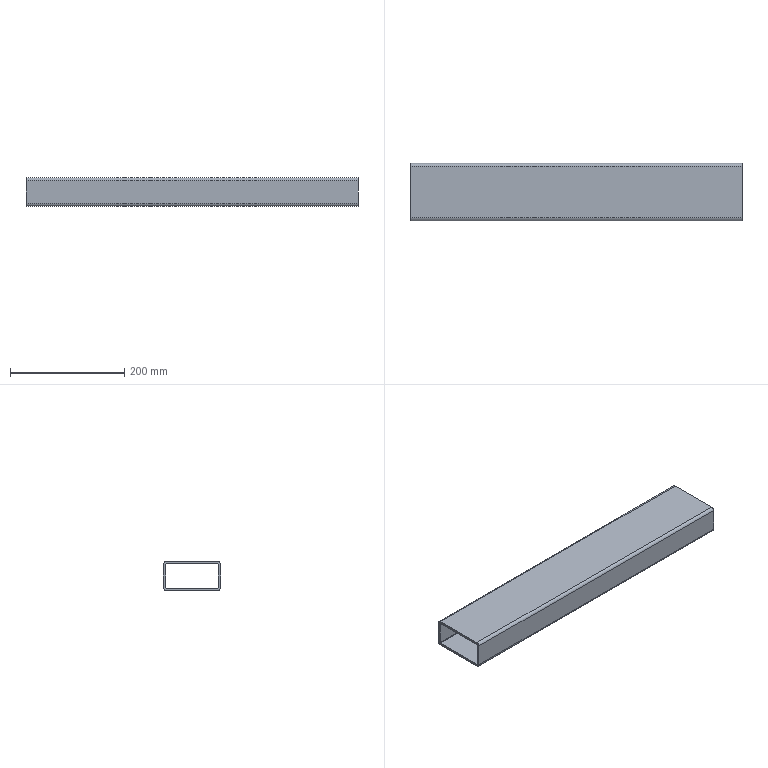Part | SolidWorks | features BaseBody 1 | 1 solid | 18 faces | box 580 x 100 x 50 mm | volume 646931 mm3 | plane 10 | cylinder 8 | commonest cylinder face diameters 2 x4 10 x4
STEP:
#1=CARTESIAN_POINT('',(-290.,45.,-25.));
#2=VERTEX_POINT('',#1);
#3=CARTESIAN_POINT('',(-290.,50.,-20.));
#4=VERTEX_POINT('',#3);
#5=CARTESIAN_POINT('',(-290.,45.,-20.));
#6=DIRECTION('',(1.,0.,0.));
#7=DIRECTION('',(0.,0.,-1.));
#8=AXIS2_PLACEMENT_3D('',#5,#6,#7);
#9=CIRCLE('',#8,5.);
#10=EDGE_CURVE('',#2,#4,#9,.T.);
#11=ORIENTED_EDGE('',*,*,#10,.T.);
#12=CARTESIAN_POINT('',(290.,50.,-20.));
#13=VERTEX_POINT('',#12);
#14=CARTESIAN_POINT('',(290.,50.,-20.));
#15=DIRECTION('',(-1.,0.,0.));
#16=VECTOR('',#15,1000.);
#17=LINE('',#14,#16);
#18=EDGE_CURVE('',#13,#4,#17,.T.);
#19=ORIENTED_EDGE('',*,*,#18,.F.);
#20=CARTESIAN_POINT('',(290.,45.,-25.));
#21=VERTEX_POINT('',#20);
#22=CARTESIAN_POINT('',(290.,45.,-20.));
#23=DIRECTION('',(1.,0.,0.));
#24=DIRECTION('',(0.,0.,-1.));
#25=AXIS2_PLACEMENT_3D('',#22,#23,#24);
#26=CIRCLE('',#25,5.);
#27=EDGE_CURVE('',#21,#13,#26,.T.);
#28=ORIENTED_EDGE('',*,*,#27,.F.);
#29=CARTESIAN_POINT('',(290.,45.,-25.));
#30=DIRECTION('',(-1.,0.,0.));
#31=VECTOR('',#30,1000.);
#32=LINE('',#29,#31);
#33=EDGE_CURVE('',#21,#2,#32,.T.);
#34=ORIENTED_EDGE('',*,*,#33,.T.);
#35=EDGE_LOOP('',(#11,#19,#28,#34));
#36=FACE_OUTER_BOUND('',#35,.T.);
#37=CARTESIAN_POINT('',(290.,45.,-20.));
#38=DIRECTION('',(-1.,0.,0.));
#39=DIRECTION('',(0.,0.,1.));
#40=AXIS2_PLACEMENT_3D('',#37,#38,#39);
#41=CYLINDRICAL_SURFACE('',#40,5.);
#42=ADVANCED_FACE('',(#36),#41,.T.);
#43=CARTESIAN_POINT('',(-290.,50.,20.));
#44=VERTEX_POINT('',#43);
#45=CARTESIAN_POINT('',(-290.,50.,-20.));
#46=DIRECTION('',(0.,0.,1.));
#47=VECTOR('',#46,1000.);
#48=LINE('',#45,#47);
#49=EDGE_CURVE('',#4,#44,#48,.T.);
#50=ORIENTED_EDGE('',*,*,#49,.T.);
#51=CARTESIAN_POINT('',(290.,50.,20.));
#52=VERTEX_POINT('',#51);
#53=CARTESIAN_POINT('',(290.,50.,20.));
#54=DIRECTION('',(-1.,0.,0.));
#55=VECTOR('',#54,1000.);
#56=LINE('',#53,#55);
#57=EDGE_CURVE('',#52,#44,#56,.T.);
#58=ORIENTED_EDGE('',*,*,#57,.F.);
#59=CARTESIAN_POINT('',(290.,50.,-20.));
#60=DIRECTION('',(0.,0.,1.));
#61=VECTOR('',#60,1000.);
#62=LINE('',#59,#61);
#63=EDGE_CURVE('',#13,#52,#62,.T.);
#64=ORIENTED_EDGE('',*,*,#63,.F.);
#65=ORIENTED_EDGE('',*,*,#18,.T.);
#66=EDGE_LOOP('',(#50,#58,#64,#65));
#67=FACE_OUTER_BOUND('',#66,.T.);
#68=CARTESIAN_POINT('',(290.,50.,-20.));
#69=DIRECTION('',(0.,-1.,0.));
#70=DIRECTION('',(0.,0.,-1.));
#71=AXIS2_PLACEMENT_3D('',#68,#69,#70);
#72=PLANE('',#71);
#73=ADVANCED_FACE('',(#67),#72,.F.);
#74=CARTESIAN_POINT('',(-290.,45.,25.));
#75=VERTEX_POINT('',#74);
#76=CARTESIAN_POINT('',(-290.,45.,20.));
#77=DIRECTION('',(1.,0.,0.));
#78=DIRECTION('',(0.,0.,-1.));
#79=AXIS2_PLACEMENT_3D('',#76,#77,#78);
#80=CIRCLE('',#79,5.);
#81=EDGE_CURVE('',#44,#75,#80,.T.);
#82=ORIENTED_EDGE('',*,*,#81,.T.);
#83=CARTESIAN_POINT('',(290.,45.,25.));
#84=VERTEX_POINT('',#83);
#85=CARTESIAN_POINT('',(290.,45.,25.));
#86=DIRECTION('',(-1.,0.,0.));
#87=VECTOR('',#86,1000.);
#88=LINE('',#85,#87);
#89=EDGE_CURVE('',#84,#75,#88,.T.);
#90=ORIENTED_EDGE('',*,*,#89,.F.);
#91=CARTESIAN_POINT('',(290.,45.,20.));
#92=DIRECTION('',(1.,0.,0.));
#93=DIRECTION('',(0.,0.,-1.));
#94=AXIS2_PLACEMENT_3D('',#91,#92,#93);
#95=CIRCLE('',#94,5.);
#96=EDGE_CURVE('',#52,#84,#95,.T.);
#97=ORIENTED_EDGE('',*,*,#96,.F.);
#98=ORIENTED_EDGE('',*,*,#57,.T.);
#99=EDGE_LOOP('',(#82,#90,#97,#98));
#100=FACE_OUTER_BOUND('',#99,.T.);
#101=CARTESIAN_POINT('',(290.,45.,20.));
#102=DIRECTION('',(-1.,0.,0.));
#103=DIRECTION('',(0.,0.,1.));
#104=AXIS2_PLACEMENT_3D('',#101,#102,#103);
#105=CYLINDRICAL_SURFACE('',#104,5.);
#106=ADVANCED_FACE('',(#100),#105,.T.);
#107=CARTESIAN_POINT('',(-290.,-45.,25.));
#108=VERTEX_POINT('',#107);
#109=CARTESIAN_POINT('',(-290.,-45.,25.));
#110=DIRECTION('',(0.,-1.,0.));
#111=VECTOR('',#110,1000.);
#112=LINE('',#109,#111);
#113=EDGE_CURVE('',#75,#108,#112,.T.);
#114=ORIENTED_EDGE('',*,*,#113,.T.);
#115=CARTESIAN_POINT('',(290.,-45.,25.));
#116=VERTEX_POINT('',#115);
#117=CARTESIAN_POINT('',(290.,-45.,25.));
#118=DIRECTION('',(-1.,0.,0.));
#119=VECTOR('',#118,1000.);
#120=LINE('',#117,#119);
#121=EDGE_CURVE('',#116,#108,#120,.T.);
#122=ORIENTED_EDGE('',*,*,#121,.F.);
#123=CARTESIAN_POINT('',(290.,-45.,25.));
#124=DIRECTION('',(0.,-1.,0.));
#125=VECTOR('',#124,1000.);
#126=LINE('',#123,#125);
#127=EDGE_CURVE('',#84,#116,#126,.T.);
#128=ORIENTED_EDGE('',*,*,#127,.F.);
#129=ORIENTED_EDGE('',*,*,#89,.T.);
#130=EDGE_LOOP('',(#114,#122,#128,#129));
#131=FACE_OUTER_BOUND('',#130,.T.);
#132=CARTESIAN_POINT('',(290.,-45.,25.));
#133=DIRECTION('',(0.,0.,-1.));
#134=DIRECTION('',(0.,1.,0.));
#135=AXIS2_PLACEMENT_3D('',#132,#133,#134);
#136=PLANE('',#135);
#137=ADVANCED_FACE('',(#131),#136,.F.);
#138=CARTESIAN_POINT('',(-290.,-50.,20.));
#139=VERTEX_POINT('',#138);
#140=CARTESIAN_POINT('',(-290.,-45.,20.));
#141=DIRECTION('',(1.,0.,0.));
#142=DIRECTION('',(0.,0.,-1.));
#143=AXIS2_PLACEMENT_3D('',#140,#141,#142);
#144=CIRCLE('',#143,5.);
#145=EDGE_CURVE('',#108,#139,#144,.T.);
#146=ORIENTED_EDGE('',*,*,#145,.T.);
#147=CARTESIAN_POINT('',(290.,-50.,20.));
#148=VERTEX_POINT('',#147);
#149=CARTESIAN_POINT('',(290.,-50.,20.));
#150=DIRECTION('',(-1.,0.,0.));
#151=VECTOR('',#150,1000.);
#152=LINE('',#149,#151);
#153=EDGE_CURVE('',#148,#139,#152,.T.);
#154=ORIENTED_EDGE('',*,*,#153,.F.);
#155=CARTESIAN_POINT('',(290.,-45.,20.));
#156=DIRECTION('',(1.,0.,0.));
#157=DIRECTION('',(0.,0.,-1.));
#158=AXIS2_PLACEMENT_3D('',#155,#156,#157);
#159=CIRCLE('',#158,5.);
#160=EDGE_CURVE('',#116,#148,#159,.T.);
#161=ORIENTED_EDGE('',*,*,#160,.F.);
#162=ORIENTED_EDGE('',*,*,#121,.T.);
#163=EDGE_LOOP('',(#146,#154,#161,#162));
#164=FACE_OUTER_BOUND('',#163,.T.);
#165=CARTESIAN_POINT('',(290.,-45.,20.));
#166=DIRECTION('',(-1.,0.,0.));
#167=DIRECTION('',(0.,0.,1.));
#168=AXIS2_PLACEMENT_3D('',#165,#166,#167);
#169=CYLINDRICAL_SURFACE('',#168,5.);
#170=ADVANCED_FACE('',(#164),#169,.T.);
#171=CARTESIAN_POINT('',(-290.,-50.,-20.));
#172=VERTEX_POINT('',#171);
#173=CARTESIAN_POINT('',(-290.,-50.,20.));
#174=DIRECTION('',(0.,0.,-1.));
#175=VECTOR('',#174,1000.);
#176=LINE('',#173,#175);
#177=EDGE_CURVE('',#139,#172,#176,.T.);
#178=ORIENTED_EDGE('',*,*,#177,.T.);
#179=CARTESIAN_POINT('',(290.,-50.,-20.));
#180=VERTEX_POINT('',#179);
#181=CARTESIAN_POINT('',(290.,-50.,-20.));
#182=DIRECTION('',(-1.,0.,0.));
#183=VECTOR('',#182,1000.);
#184=LINE('',#181,#183);
#185=EDGE_CURVE('',#180,#172,#184,.T.);
#186=ORIENTED_EDGE('',*,*,#185,.F.);
#187=CARTESIAN_POINT('',(290.,-50.,20.));
#188=DIRECTION('',(0.,0.,-1.));
#189=VECTOR('',#188,1000.);
#190=LINE('',#187,#189);
#191=EDGE_CURVE('',#148,#180,#190,.T.);
#192=ORIENTED_EDGE('',*,*,#191,.F.);
#193=ORIENTED_EDGE('',*,*,#153,.T.);
#194=EDGE_LOOP('',(#178,#186,#192,#193));
#195=FACE_OUTER_BOUND('',#194,.T.);
#196=CARTESIAN_POINT('',(290.,-50.,20.));
#197=DIRECTION('',(0.,1.,0.));
#198=DIRECTION('',(0.,0.,1.));
#199=AXIS2_PLACEMENT_3D('',#196,#197,#198);
#200=PLANE('',#199);
#201=ADVANCED_FACE('',(#195),#200,.F.);
#202=CARTESIAN_POINT('',(-290.,-45.,-25.));
#203=VERTEX_POINT('',#202);
#204=CARTESIAN_POINT('',(-290.,-45.,-20.));
#205=DIRECTION('',(1.,0.,0.));
#206=DIRECTION('',(0.,0.,-1.));
#207=AXIS2_PLACEMENT_3D('',#204,#205,#206);
#208=CIRCLE('',#207,5.);
#209=EDGE_CURVE('',#172,#203,#208,.T.);
#210=ORIENTED_EDGE('',*,*,#209,.T.);
#211=CARTESIAN_POINT('',(290.,-45.,-25.));
#212=VERTEX_POINT('',#211);
#213=CARTESIAN_POINT('',(290.,-45.,-25.));
#214=DIRECTION('',(-1.,0.,0.));
#215=VECTOR('',#214,1000.);
#216=LINE('',#213,#215);
#217=EDGE_CURVE('',#212,#203,#216,.T.);
#218=ORIENTED_EDGE('',*,*,#217,.F.);
#219=CARTESIAN_POINT('',(290.,-45.,-20.));
#220=DIRECTION('',(1.,0.,0.));
#221=DIRECTION('',(0.,0.,-1.));
#222=AXIS2_PLACEMENT_3D('',#219,#220,#221);
#223=CIRCLE('',#222,5.);
#224=EDGE_CURVE('',#180,#212,#223,.T.);
#225=ORIENTED_EDGE('',*,*,#224,.F.);
#226=ORIENTED_EDGE('',*,*,#185,.T.);
#227=EDGE_LOOP('',(#210,#218,#225,#226));
#228=FACE_OUTER_BOUND('',#227,.T.);
#229=CARTESIAN_POINT('',(290.,-45.,-20.));
#230=DIRECTION('',(-1.,0.,0.));
#231=DIRECTION('',(0.,0.,1.));
#232=AXIS2_PLACEMENT_3D('',#229,#230,#231);
#233=CYLINDRICAL_SURFACE('',#232,5.);
#234=ADVANCED_FACE('',(#228),#233,.T.);
#235=CARTESIAN_POINT('',(-290.,46.,20.));
#236=VERTEX_POINT('',#235);
#237=CARTESIAN_POINT('',(-290.,45.,21.));
#238=VERTEX_POINT('',#237);
#239=CARTESIAN_POINT('',(-290.,45.,20.));
#240=DIRECTION('',(1.,0.,0.));
#241=DIRECTION('',(0.,0.,-1.));
#242=AXIS2_PLACEMENT_3D('',#239,#240,#241);
#243=CIRCLE('',#242,1.);
#244=EDGE_CURVE('',#236,#238,#243,.T.);
#245=ORIENTED_EDGE('',*,*,#244,.F.);
#246=CARTESIAN_POINT('',(290.,46.,20.));
#247=VERTEX_POINT('',#246);
#248=CARTESIAN_POINT('',(290.,46.,20.));
#249=DIRECTION('',(-1.,0.,0.));
#250=VECTOR('',#249,1000.);
#251=LINE('',#248,#250);
#252=EDGE_CURVE('',#247,#236,#251,.T.);
#253=ORIENTED_EDGE('',*,*,#252,.F.);
#254=CARTESIAN_POINT('',(290.,45.,21.));
#255=VERTEX_POINT('',#254);
#256=CARTESIAN_POINT('',(290.,45.,20.));
#257=DIRECTION('',(1.,0.,0.));
#258=DIRECTION('',(0.,0.,-1.));
#259=AXIS2_PLACEMENT_3D('',#256,#257,#258);
#260=CIRCLE('',#259,1.);
#261=EDGE_CURVE('',#247,#255,#260,.T.);
#262=ORIENTED_EDGE('',*,*,#261,.T.);
#263=CARTESIAN_POINT('',(290.,45.,21.));
#264=DIRECTION('',(-1.,0.,0.));
#265=VECTOR('',#264,1000.);
#266=LINE('',#263,#265);
#267=EDGE_CURVE('',#255,#238,#266,.T.);
#268=ORIENTED_EDGE('',*,*,#267,.T.);
#269=EDGE_LOOP('',(#245,#253,#262,#268));
#270=FACE_OUTER_BOUND('',#269,.T.);
#271=CARTESIAN_POINT('',(290.,45.,20.));
#272=DIRECTION('',(-1.,0.,0.));
#273=DIRECTION('',(0.,0.,1.));
#274=AXIS2_PLACEMENT_3D('',#271,#272,#273);
#275=CYLINDRICAL_SURFACE('',#274,1.);
#276=ADVANCED_FACE('',(#270),#275,.F.);
#277=CARTESIAN_POINT('',(-290.,46.,-20.));
#278=VERTEX_POINT('',#277);
#279=CARTESIAN_POINT('',(-290.,46.,-20.));
#280=DIRECTION('',(0.,0.,1.));
#281=VECTOR('',#280,1000.);
#282=LINE('',#279,#281);
#283=EDGE_CURVE('',#278,#236,#282,.T.);
#284=ORIENTED_EDGE('',*,*,#283,.F.);
#285=CARTESIAN_POINT('',(290.,46.,-20.));
#286=VERTEX_POINT('',#285);
#287=CARTESIAN_POINT('',(290.,46.,-20.));
#288=DIRECTION('',(-1.,0.,0.));
#289=VECTOR('',#288,1000.);
#290=LINE('',#287,#289);
#291=EDGE_CURVE('',#286,#278,#290,.T.);
#292=ORIENTED_EDGE('',*,*,#291,.F.);
#293=CARTESIAN_POINT('',(290.,46.,-20.));
#294=DIRECTION('',(0.,0.,1.));
#295=VECTOR('',#294,1000.);
#296=LINE('',#293,#295);
#297=EDGE_CURVE('',#286,#247,#296,.T.);
#298=ORIENTED_EDGE('',*,*,#297,.T.);
#299=ORIENTED_EDGE('',*,*,#252,.T.);
#300=EDGE_LOOP('',(#284,#292,#298,#299));
#301=FACE_OUTER_BOUND('',#300,.T.);
#302=CARTESIAN_POINT('',(290.,46.,-20.));
#303=DIRECTION('',(0.,-1.,0.));
#304=DIRECTION('',(0.,0.,-1.));
#305=AXIS2_PLACEMENT_3D('',#302,#303,#304);
#306=PLANE('',#305);
#307=ADVANCED_FACE('',(#301),#306,.T.);
#308=CARTESIAN_POINT('',(-290.,45.,-21.));
#309=VERTEX_POINT('',#308);
#310=CARTESIAN_POINT('',(-290.,45.,-20.));
#311=DIRECTION('',(1.,0.,0.));
#312=DIRECTION('',(0.,0.,-1.));
#313=AXIS2_PLACEMENT_3D('',#310,#311,#312);
#314=CIRCLE('',#313,1.);
#315=EDGE_CURVE('',#309,#278,#314,.T.);
#316=ORIENTED_EDGE('',*,*,#315,.F.);
#317=CARTESIAN_POINT('',(290.,45.,-21.));
#318=VERTEX_POINT('',#317);
#319=CARTESIAN_POINT('',(290.,45.,-21.));
#320=DIRECTION('',(-1.,0.,0.));
#321=VECTOR('',#320,1000.);
#322=LINE('',#319,#321);
#323=EDGE_CURVE('',#318,#309,#322,.T.);
#324=ORIENTED_EDGE('',*,*,#323,.F.);
#325=CARTESIAN_POINT('',(290.,45.,-20.));
#326=DIRECTION('',(1.,0.,0.));
#327=DIRECTION('',(0.,0.,-1.));
#328=AXIS2_PLACEMENT_3D('',#325,#326,#327);
#329=CIRCLE('',#328,1.);
#330=EDGE_CURVE('',#318,#286,#329,.T.);
#331=ORIENTED_EDGE('',*,*,#330,.T.);
#332=ORIENTED_EDGE('',*,*,#291,.T.);
#333=EDGE_LOOP('',(#316,#324,#331,#332));
#334=FACE_OUTER_BOUND('',#333,.T.);
#335=CARTESIAN_POINT('',(290.,45.,-20.));
#336=DIRECTION('',(-1.,0.,0.));
#337=DIRECTION('',(0.,0.,1.));
#338=AXIS2_PLACEMENT_3D('',#335,#336,#337);
#339=CYLINDRICAL_SURFACE('',#338,1.);
#340=ADVANCED_FACE('',(#334),#339,.F.);
#341=CARTESIAN_POINT('',(-290.,-45.,-21.));
#342=VERTEX_POINT('',#341);
#343=CARTESIAN_POINT('',(-290.,45.,-21.));
#344=DIRECTION('',(0.,1.,0.));
#345=VECTOR('',#344,1000.);
#346=LINE('',#343,#345);
#347=EDGE_CURVE('',#342,#309,#346,.T.);
#348=ORIENTED_EDGE('',*,*,#347,.F.);
#349=CARTESIAN_POINT('',(290.,-45.,-21.));
#350=VERTEX_POINT('',#349);
#351=CARTESIAN_POINT('',(290.,-45.,-21.));
#352=DIRECTION('',(-1.,0.,0.));
#353=VECTOR('',#352,1000.);
#354=LINE('',#351,#353);
#355=EDGE_CURVE('',#350,#342,#354,.T.);
#356=ORIENTED_EDGE('',*,*,#355,.F.);
#357=CARTESIAN_POINT('',(290.,45.,-21.));
#358=DIRECTION('',(0.,1.,0.));
#359=VECTOR('',#358,1000.);
#360=LINE('',#357,#359);
#361=EDGE_CURVE('',#350,#318,#360,.T.);
#362=ORIENTED_EDGE('',*,*,#361,.T.);
#363=ORIENTED_EDGE('',*,*,#323,.T.);
#364=EDGE_LOOP('',(#348,#356,#362,#363));
#365=FACE_OUTER_BOUND('',#364,.T.);
#366=CARTESIAN_POINT('',(290.,45.,-21.));
#367=DIRECTION('',(0.,0.,1.));
#368=DIRECTION('',(1.,0.,0.));
#369=AXIS2_PLACEMENT_3D('',#366,#367,#368);
#370=PLANE('',#369);
#371=ADVANCED_FACE('',(#365),#370,.T.);
#372=CARTESIAN_POINT('',(-290.,-46.,-20.));
#373=VERTEX_POINT('',#372);
#374=CARTESIAN_POINT('',(-290.,-45.,-20.));
#375=DIRECTION('',(1.,0.,0.));
#376=DIRECTION('',(0.,0.,-1.));
#377=AXIS2_PLACEMENT_3D('',#374,#375,#376);
#378=CIRCLE('',#377,1.);
#379=EDGE_CURVE('',#373,#342,#378,.T.);
#380=ORIENTED_EDGE('',*,*,#379,.F.);
#381=CARTESIAN_POINT('',(290.,-46.,-20.));
#382=VERTEX_POINT('',#381);
#383=CARTESIAN_POINT('',(290.,-46.,-20.));
#384=DIRECTION('',(-1.,0.,0.));
#385=VECTOR('',#384,1000.);
#386=LINE('',#383,#385);
#387=EDGE_CURVE('',#382,#373,#386,.T.);
#388=ORIENTED_EDGE('',*,*,#387,.F.);
#389=CARTESIAN_POINT('',(290.,-45.,-20.));
#390=DIRECTION('',(1.,0.,0.));
#391=DIRECTION('',(0.,0.,-1.));
#392=AXIS2_PLACEMENT_3D('',#389,#390,#391);
#393=CIRCLE('',#392,1.);
#394=EDGE_CURVE('',#382,#350,#393,.T.);
#395=ORIENTED_EDGE('',*,*,#394,.T.);
#396=ORIENTED_EDGE('',*,*,#355,.T.);
#397=EDGE_LOOP('',(#380,#388,#395,#396));
#398=FACE_OUTER_BOUND('',#397,.T.);
#399=CARTESIAN_POINT('',(290.,-45.,-20.));
#400=DIRECTION('',(-1.,0.,0.));
#401=DIRECTION('',(0.,0.,1.));
#402=AXIS2_PLACEMENT_3D('',#399,#400,#401);
#403=CYLINDRICAL_SURFACE('',#402,1.);
#404=ADVANCED_FACE('',(#398),#403,.F.);
#405=CARTESIAN_POINT('',(-290.,-46.,20.));
#406=VERTEX_POINT('',#405);
#407=CARTESIAN_POINT('',(-290.,-46.,20.));
#408=DIRECTION('',(0.,0.,-1.));
#409=VECTOR('',#408,1000.);
#410=LINE('',#407,#409);
#411=EDGE_CURVE('',#406,#373,#410,.T.);
#412=ORIENTED_EDGE('',*,*,#411,.F.);
#413=CARTESIAN_POINT('',(290.,-46.,20.));
#414=VERTEX_POINT('',#413);
#415=CARTESIAN_POINT('',(290.,-46.,20.));
#416=DIRECTION('',(-1.,0.,0.));
#417=VECTOR('',#416,1000.);
#418=LINE('',#415,#417);
#419=EDGE_CURVE('',#414,#406,#418,.T.);
#420=ORIENTED_EDGE('',*,*,#419,.F.);
#421=CARTESIAN_POINT('',(290.,-46.,20.));
#422=DIRECTION('',(0.,0.,-1.));
#423=VECTOR('',#422,1000.);
#424=LINE('',#421,#423);
#425=EDGE_CURVE('',#414,#382,#424,.T.);
#426=ORIENTED_EDGE('',*,*,#425,.T.);
#427=ORIENTED_EDGE('',*,*,#387,.T.);
#428=EDGE_LOOP('',(#412,#420,#426,#427));
#429=FACE_OUTER_BOUND('',#428,.T.);
#430=CARTESIAN_POINT('',(290.,-46.,20.));
#431=DIRECTION('',(0.,1.,0.));
#432=DIRECTION('',(0.,0.,1.));
#433=AXIS2_PLACEMENT_3D('',#430,#431,#432);
#434=PLANE('',#433);
#435=ADVANCED_FACE('',(#429),#434,.T.);
#436=CARTESIAN_POINT('',(-290.,-45.,21.));
#437=VERTEX_POINT('',#436);
#438=CARTESIAN_POINT('',(-290.,-45.,20.));
#439=DIRECTION('',(1.,0.,0.));
#440=DIRECTION('',(0.,0.,-1.));
#441=AXIS2_PLACEMENT_3D('',#438,#439,#440);
#442=CIRCLE('',#441,1.);
#443=EDGE_CURVE('',#437,#406,#442,.T.);
#444=ORIENTED_EDGE('',*,*,#443,.F.);
#445=CARTESIAN_POINT('',(290.,-45.,21.));
#446=VERTEX_POINT('',#445);
#447=CARTESIAN_POINT('',(290.,-45.,21.));
#448=DIRECTION('',(-1.,0.,0.));
#449=VECTOR('',#448,1000.);
#450=LINE('',#447,#449);
#451=EDGE_CURVE('',#446,#437,#450,.T.);
#452=ORIENTED_EDGE('',*,*,#451,.F.);
#453=CARTESIAN_POINT('',(290.,-45.,20.));
#454=DIRECTION('',(1.,0.,0.));
#455=DIRECTION('',(0.,0.,-1.));
#456=AXIS2_PLACEMENT_3D('',#453,#454,#455);
#457=CIRCLE('',#456,1.);
#458=EDGE_CURVE('',#446,#414,#457,.T.);
#459=ORIENTED_EDGE('',*,*,#458,.T.);
#460=ORIENTED_EDGE('',*,*,#419,.T.);
#461=EDGE_LOOP('',(#444,#452,#459,#460));
#462=FACE_OUTER_BOUND('',#461,.T.);
#463=CARTESIAN_POINT('',(290.,-45.,20.));
#464=DIRECTION('',(-1.,0.,0.));
#465=DIRECTION('',(0.,0.,1.));
#466=AXIS2_PLACEMENT_3D('',#463,#464,#465);
#467=CYLINDRICAL_SURFACE('',#466,1.);
#468=ADVANCED_FACE('',(#462),#467,.F.);
#469=CARTESIAN_POINT('',(-290.,-45.,21.));
#470=DIRECTION('',(0.,-1.,0.));
#471=VECTOR('',#470,1000.);
#472=LINE('',#469,#471);
#473=EDGE_CURVE('',#238,#437,#472,.T.);
#474=ORIENTED_EDGE('',*,*,#473,.F.);
#475=ORIENTED_EDGE('',*,*,#267,.F.);
#476=CARTESIAN_POINT('',(290.,-45.,21.));
#477=DIRECTION('',(0.,-1.,0.));
#478=VECTOR('',#477,1000.);
#479=LINE('',#476,#478);
#480=EDGE_CURVE('',#255,#446,#479,.T.);
#481=ORIENTED_EDGE('',*,*,#480,.T.);
#482=ORIENTED_EDGE('',*,*,#451,.T.);
#483=EDGE_LOOP('',(#474,#475,#481,#482));
#484=FACE_OUTER_BOUND('',#483,.T.);
#485=CARTESIAN_POINT('',(290.,-45.,21.));
#486=DIRECTION('',(0.,0.,-1.));
#487=DIRECTION('',(0.,1.,0.));
#488=AXIS2_PLACEMENT_3D('',#485,#486,#487);
#489=PLANE('',#488);
#490=ADVANCED_FACE('',(#484),#489,.T.);
#491=CARTESIAN_POINT('',(-290.,45.,-25.));
#492=DIRECTION('',(0.,1.,0.));
#493=VECTOR('',#492,1000.);
#494=LINE('',#491,#493);
#495=EDGE_CURVE('',#203,#2,#494,.T.);
#496=ORIENTED_EDGE('',*,*,#495,.T.);
#497=ORIENTED_EDGE('',*,*,#33,.F.);
#498=CARTESIAN_POINT('',(290.,45.,-25.));
#499=DIRECTION('',(0.,1.,0.));
#500=VECTOR('',#499,1000.);
#501=LINE('',#498,#500);
#502=EDGE_CURVE('',#212,#21,#501,.T.);
#503=ORIENTED_EDGE('',*,*,#502,.F.);
#504=ORIENTED_EDGE('',*,*,#217,.T.);
#505=EDGE_LOOP('',(#496,#497,#503,#504));
#506=FACE_OUTER_BOUND('',#505,.T.);
#507=CARTESIAN_POINT('',(290.,45.,-25.));
#508=DIRECTION('',(0.,0.,1.));
#509=DIRECTION('',(1.,0.,0.));
#510=AXIS2_PLACEMENT_3D('',#507,#508,#509);
#511=PLANE('',#510);
#512=ADVANCED_FACE('',(#506),#511,.F.);
#513=ORIENTED_EDGE('',*,*,#261,.F.);
#514=ORIENTED_EDGE('',*,*,#297,.F.);
#515=ORIENTED_EDGE('',*,*,#330,.F.);
#516=ORIENTED_EDGE('',*,*,#361,.F.);
#517=ORIENTED_EDGE('',*,*,#394,.F.);
#518=ORIENTED_EDGE('',*,*,#425,.F.);
#519=ORIENTED_EDGE('',*,*,#458,.F.);
#520=ORIENTED_EDGE('',*,*,#480,.F.);
#521=EDGE_LOOP('',(#513,#514,#515,#516,#517,#518,#519,#520));
#522=FACE_BOUND('',#521,.T.);
#523=ORIENTED_EDGE('',*,*,#27,.T.);
#524=ORIENTED_EDGE('',*,*,#63,.T.);
#525=ORIENTED_EDGE('',*,*,#96,.T.);
#526=ORIENTED_EDGE('',*,*,#127,.T.);
#527=ORIENTED_EDGE('',*,*,#160,.T.);
#528=ORIENTED_EDGE('',*,*,#191,.T.);
#529=ORIENTED_EDGE('',*,*,#224,.T.);
#530=ORIENTED_EDGE('',*,*,#502,.T.);
#531=EDGE_LOOP('',(#523,#524,#525,#526,#527,#528,#529,#530));
#532=FACE_OUTER_BOUND('',#531,.T.);
#533=CARTESIAN_POINT('',(290.,45.,-20.));
#534=DIRECTION('',(1.,0.,0.));
#535=DIRECTION('',(0.,0.,-1.));
#536=AXIS2_PLACEMENT_3D('',#533,#534,#535);
#537=PLANE('',#536);
#538=ADVANCED_FACE('',(#522,#532),#537,.T.);
#539=ORIENTED_EDGE('',*,*,#244,.T.);
#540=ORIENTED_EDGE('',*,*,#473,.T.);
#541=ORIENTED_EDGE('',*,*,#443,.T.);
#542=ORIENTED_EDGE('',*,*,#411,.T.);
#543=ORIENTED_EDGE('',*,*,#379,.T.);
#544=ORIENTED_EDGE('',*,*,#347,.T.);
#545=ORIENTED_EDGE('',*,*,#315,.T.);
#546=ORIENTED_EDGE('',*,*,#283,.T.);
#547=EDGE_LOOP('',(#539,#540,#541,#542,#543,#544,#545,#546));
#548=FACE_BOUND('',#547,.T.);
#549=ORIENTED_EDGE('',*,*,#10,.F.);
#550=ORIENTED_EDGE('',*,*,#495,.F.);
#551=ORIENTED_EDGE('',*,*,#209,.F.);
#552=ORIENTED_EDGE('',*,*,#177,.F.);
#553=ORIENTED_EDGE('',*,*,#145,.F.);
#554=ORIENTED_EDGE('',*,*,#113,.F.);
#555=ORIENTED_EDGE('',*,*,#81,.F.);
#556=ORIENTED_EDGE('',*,*,#49,.F.);
#557=EDGE_LOOP('',(#549,#550,#551,#552,#553,#554,#555,#556));
#558=FACE_OUTER_BOUND('',#557,.T.);
#559=CARTESIAN_POINT('',(-290.,45.,-20.));
#560=DIRECTION('',(1.,0.,0.));
#561=DIRECTION('',(0.,0.,-1.));
#562=AXIS2_PLACEMENT_3D('',#559,#560,#561);
#563=PLANE('',#562);
#564=ADVANCED_FACE('',(#548,#558),#563,.F.);
#565=CLOSED_SHELL('',(#42,#73,#106,#137,#170,#201,#234,#276,#307,#340,#371,#404,#435,#468,#490,#512,#538,#564));
#566=MANIFOLD_SOLID_BREP('',#565);
#567=CARTESIAN_POINT('',(0.,0.,0.));
#568=DIRECTION('',(0.,0.,1.));
#569=DIRECTION('',(1.,0.,0.));
#570=AXIS2_PLACEMENT_3D('',#567,#568,#569);
#571=(LENGTH_UNIT()NAMED_UNIT(*)SI_UNIT(.MILLI.,.METRE.));
#572=UNCERTAINTY_MEASURE_WITH_UNIT(LENGTH_MEASURE(0.00001),#571,'','');
#573=(NAMED_UNIT(*)PLANE_ANGLE_UNIT()SI_UNIT($,.RADIAN.));
#574=(NAMED_UNIT(*)SI_UNIT($,.STERADIAN.)SOLID_ANGLE_UNIT());
#575=(GEOMETRIC_REPRESENTATION_CONTEXT(3)GLOBAL_UNCERTAINTY_ASSIGNED_CONTEXT((#572))GLOBAL_UNIT_ASSIGNED_CONTEXT((#571,#573,#574))REPRESENTATION_CONTEXT('',''));
#576=ADVANCED_BREP_SHAPE_REPRESENTATION('',(#566,#570),#575);